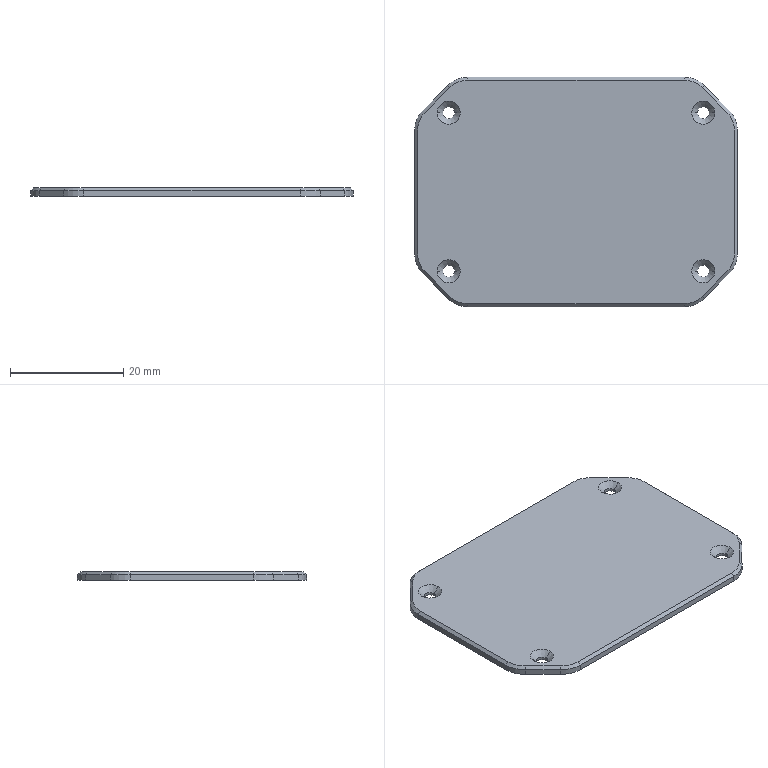Part | 1 solid | 62 faces | box 57 x 40.5 x 1.5 mm | volume 3226 mm3 | cylinder 24 | plane 22 | cone 16 | commonest cylinder face diameters 2.1 x8 4.5 x8 10 x8